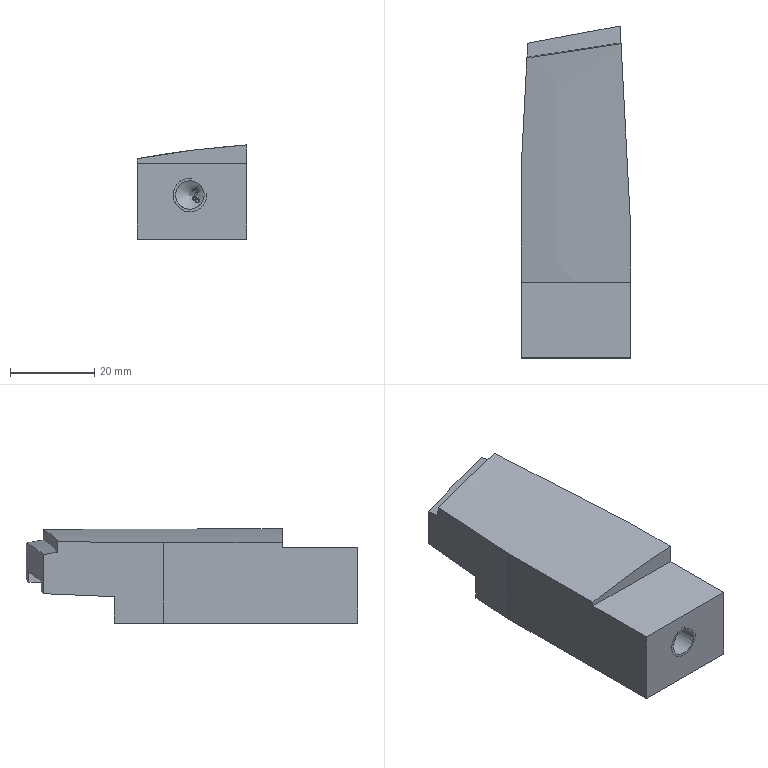Part | STEP file | P011002S004-002 | 1 solid | 52 faces | box 26 x 79.009 x 22.435 mm | volume 34276 mm3 | plane 29 | other 11 | cone 7 | cylinder 3 | spline 2 | commonest cylinder face diameters 6.8 x1 7.973 x1 8 x1